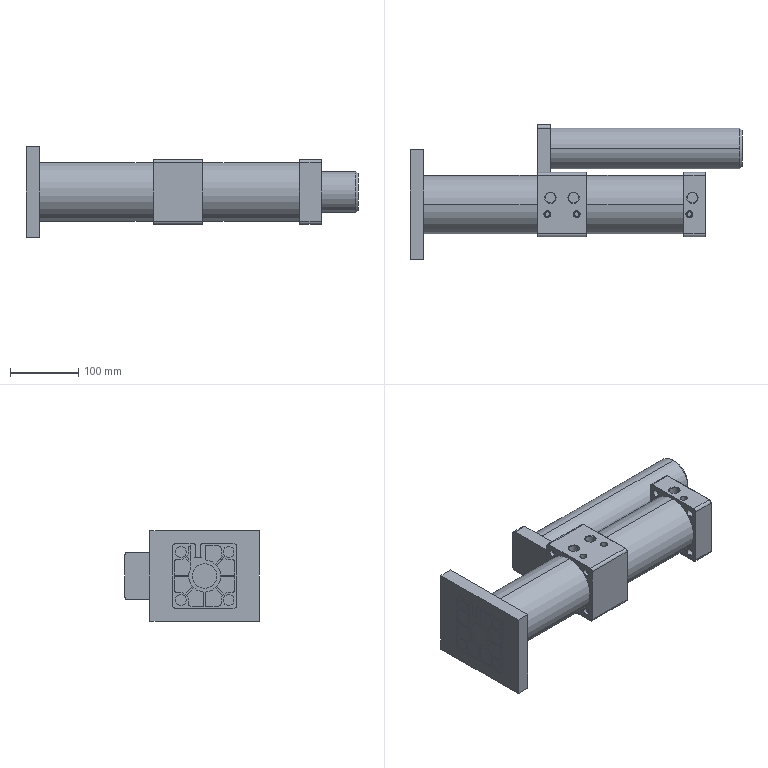Part | STEP file | SCT_80x100x25_c | 3 solids | 438 faces | box 486 x 197 x 132 mm | volume 2272185 mm3 | cylinder 194 | plane 179 | cone 63 | torus 2 | commonest cylinder face diameters 10.5 x32 8 x31 16 x21 7 x16 8.376 x16 22 x12